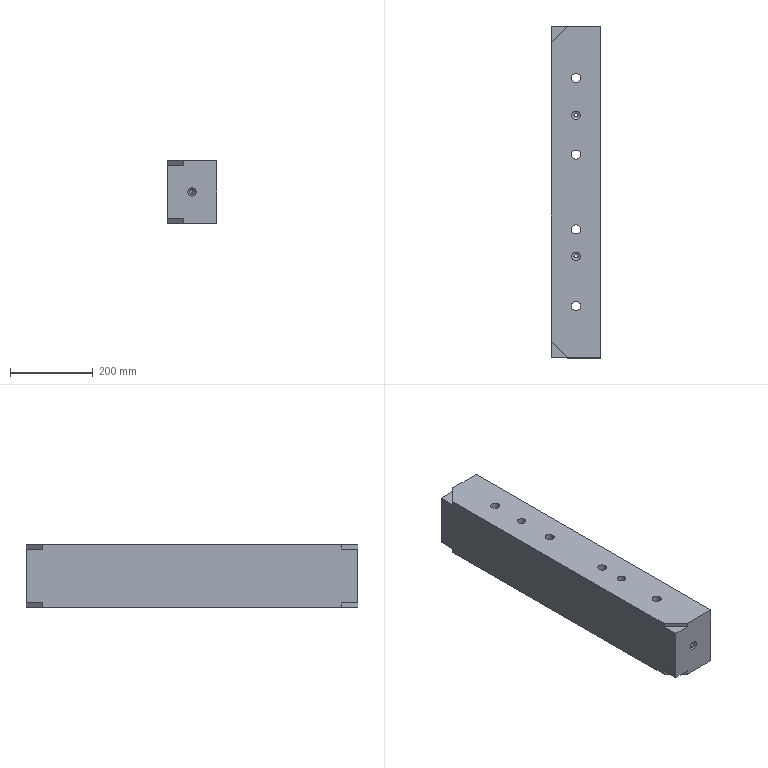Part | Creo | 1 solid | 62 faces | box 120 x 800 x 150 mm | volume 14066670 mm3 | cylinder 28 | cone 20 | plane 14 | commonest cylinder face diameters 20 x8 22 x8 8 x4 12 x4 14 x4